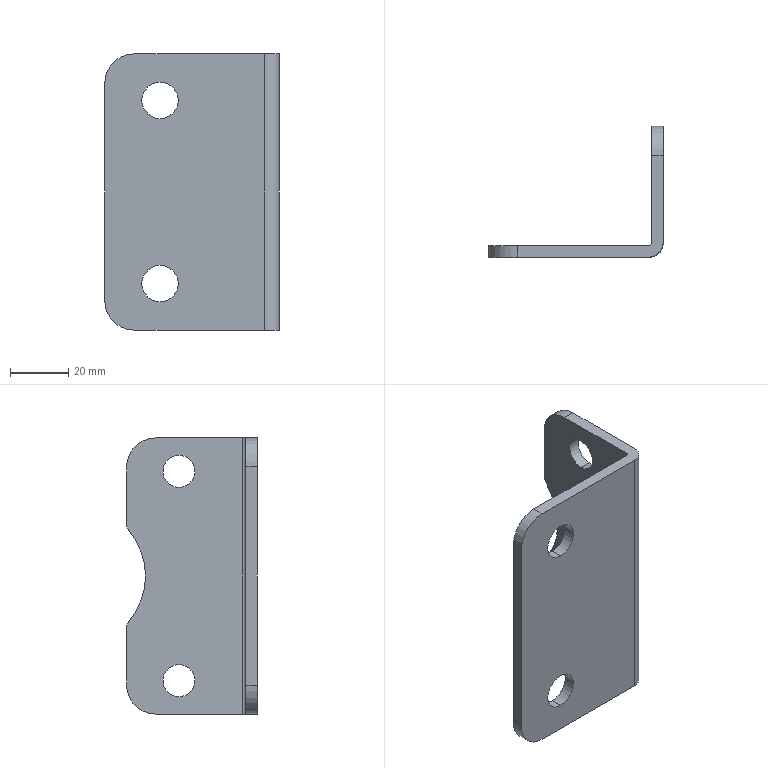Part | NX | features BREP 1 | 1 solid | 26 faces | box 60 x 45 x 95 mm | volume 35211 mm3 | cylinder 17 | plane 9 | commonest cylinder face diameters 11 x4 12.5 x4 20 x4 4 x2 2 x1 10 x1
STEP:
#1=CARTESIAN_POINT('',(-41.,-63.,-37.75));
#2=VERTEX_POINT('',#1);
#3=CARTESIAN_POINT('',(-41.,-63.,-25.25));
#4=VERTEX_POINT('',#3);
#5=CARTESIAN_POINT('',(-41.,-63.,-31.5));
#6=DIRECTION('',(0.,1.,0.));
#7=DIRECTION('',(0.,0.,1.));
#8=AXIS2_PLACEMENT_3D('',#5,#6,#7);
#9=CIRCLE('',#8,6.25);
#10=EDGE_CURVE('',#2,#4,#9,.T.);
#11=ORIENTED_EDGE('',*,*,#10,.F.);
#12=CARTESIAN_POINT('',(-41.,-59.,-37.75));
#13=VERTEX_POINT('',#12);
#14=CARTESIAN_POINT('',(-41.,-59.,-37.75));
#15=DIRECTION('',(0.,1.,0.));
#16=VECTOR('',#15,1000.);
#17=LINE('',#14,#16);
#18=EDGE_CURVE('',#13,#2,#17,.F.);
#19=ORIENTED_EDGE('',*,*,#18,.F.);
#20=CARTESIAN_POINT('',(-41.,-59.,-25.25));
#21=VERTEX_POINT('',#20);
#22=CARTESIAN_POINT('',(-41.,-59.,-31.5));
#23=DIRECTION('',(0.,1.,0.));
#24=DIRECTION('',(0.,0.,1.));
#25=AXIS2_PLACEMENT_3D('',#22,#23,#24);
#26=CIRCLE('',#25,6.25);
#27=EDGE_CURVE('',#13,#21,#26,.T.);
#28=ORIENTED_EDGE('',*,*,#27,.T.);
#29=CARTESIAN_POINT('',(-41.,-59.,-25.25));
#30=DIRECTION('',(0.,1.,0.));
#31=VECTOR('',#30,1000.);
#32=LINE('',#29,#31);
#33=EDGE_CURVE('',#21,#4,#32,.F.);
#34=ORIENTED_EDGE('',*,*,#33,.T.);
#35=EDGE_LOOP('',(#11,#19,#28,#34));
#36=FACE_BOUND('',#35,.T.);
#37=CARTESIAN_POINT('',(-41.,-59.,-31.5));
#38=DIRECTION('',(0.,1.,0.));
#39=DIRECTION('',(0.,0.,1.));
#40=AXIS2_PLACEMENT_3D('',#37,#38,#39);
#41=CYLINDRICAL_SURFACE('',#40,6.25);
#42=ADVANCED_FACE('',(#36),#41,.F.);
#43=CARTESIAN_POINT('',(-41.,-63.,25.25));
#44=VERTEX_POINT('',#43);
#45=CARTESIAN_POINT('',(-41.,-63.,37.75));
#46=VERTEX_POINT('',#45);
#47=CARTESIAN_POINT('',(-41.,-63.,31.5));
#48=DIRECTION('',(0.,1.,0.));
#49=DIRECTION('',(0.,0.,1.));
#50=AXIS2_PLACEMENT_3D('',#47,#48,#49);
#51=CIRCLE('',#50,6.25);
#52=EDGE_CURVE('',#44,#46,#51,.T.);
#53=ORIENTED_EDGE('',*,*,#52,.F.);
#54=CARTESIAN_POINT('',(-41.,-59.,25.25));
#55=VERTEX_POINT('',#54);
#56=CARTESIAN_POINT('',(-41.,-59.,25.25));
#57=DIRECTION('',(0.,1.,0.));
#58=VECTOR('',#57,1000.);
#59=LINE('',#56,#58);
#60=EDGE_CURVE('',#55,#44,#59,.F.);
#61=ORIENTED_EDGE('',*,*,#60,.F.);
#62=CARTESIAN_POINT('',(-41.,-59.,37.75));
#63=VERTEX_POINT('',#62);
#64=CARTESIAN_POINT('',(-41.,-59.,31.5));
#65=DIRECTION('',(0.,1.,0.));
#66=DIRECTION('',(0.,0.,1.));
#67=AXIS2_PLACEMENT_3D('',#64,#65,#66);
#68=CIRCLE('',#67,6.25);
#69=EDGE_CURVE('',#55,#63,#68,.T.);
#70=ORIENTED_EDGE('',*,*,#69,.T.);
#71=CARTESIAN_POINT('',(-41.,-59.,37.75));
#72=DIRECTION('',(0.,1.,0.));
#73=VECTOR('',#72,1000.);
#74=LINE('',#71,#73);
#75=EDGE_CURVE('',#63,#46,#74,.F.);
#76=ORIENTED_EDGE('',*,*,#75,.T.);
#77=EDGE_LOOP('',(#53,#61,#70,#76));
#78=FACE_BOUND('',#77,.T.);
#79=CARTESIAN_POINT('',(-41.,-59.,31.5));
#80=DIRECTION('',(0.,1.,0.));
#81=DIRECTION('',(0.,0.,1.));
#82=AXIS2_PLACEMENT_3D('',#79,#80,#81);
#83=CYLINDRICAL_SURFACE('',#82,6.25);
#84=ADVANCED_FACE('',(#78),#83,.F.);
#85=CARTESIAN_POINT('',(-4.,-36.,-41.5));
#86=VERTEX_POINT('',#85);
#87=CARTESIAN_POINT('',(-4.,-36.,-30.5));
#88=VERTEX_POINT('',#87);
#89=CARTESIAN_POINT('',(-4.,-36.,-36.));
#90=DIRECTION('',(-1.,0.,0.));
#91=DIRECTION('',(0.,0.,-1.));
#92=AXIS2_PLACEMENT_3D('',#89,#90,#91);
#93=CIRCLE('',#92,5.5);
#94=EDGE_CURVE('',#86,#88,#93,.T.);
#95=ORIENTED_EDGE('',*,*,#94,.T.);
#96=CARTESIAN_POINT('',(0.,-36.,-30.5));
#97=VERTEX_POINT('',#96);
#98=CARTESIAN_POINT('',(4.,-36.,-30.5));
#99=DIRECTION('',(1.,0.,0.));
#100=VECTOR('',#99,1000.);
#101=LINE('',#98,#100);
#102=EDGE_CURVE('',#88,#97,#101,.T.);
#103=ORIENTED_EDGE('',*,*,#102,.T.);
#104=CARTESIAN_POINT('',(0.,-36.,-41.5));
#105=VERTEX_POINT('',#104);
#106=CARTESIAN_POINT('',(0.,-36.,-36.));
#107=DIRECTION('',(1.,0.,0.));
#108=DIRECTION('',(0.,0.,-1.));
#109=AXIS2_PLACEMENT_3D('',#106,#107,#108);
#110=CIRCLE('',#109,5.5);
#111=EDGE_CURVE('',#97,#105,#110,.T.);
#112=ORIENTED_EDGE('',*,*,#111,.T.);
#113=CARTESIAN_POINT('',(4.,-36.,-41.5));
#114=DIRECTION('',(1.,0.,0.));
#115=VECTOR('',#114,1000.);
#116=LINE('',#113,#115);
#117=EDGE_CURVE('',#86,#105,#116,.T.);
#118=ORIENTED_EDGE('',*,*,#117,.F.);
#119=EDGE_LOOP('',(#95,#103,#112,#118));
#120=FACE_BOUND('',#119,.T.);
#121=CARTESIAN_POINT('',(4.,-36.,-36.));
#122=DIRECTION('',(1.,0.,0.));
#123=DIRECTION('',(0.,0.,-1.));
#124=AXIS2_PLACEMENT_3D('',#121,#122,#123);
#125=CYLINDRICAL_SURFACE('',#124,5.5);
#126=ADVANCED_FACE('',(#120),#125,.F.);
#127=CARTESIAN_POINT('',(-4.,-36.,30.5));
#128=VERTEX_POINT('',#127);
#129=CARTESIAN_POINT('',(-4.,-36.,41.5));
#130=VERTEX_POINT('',#129);
#131=CARTESIAN_POINT('',(-4.,-36.,36.));
#132=DIRECTION('',(-1.,0.,0.));
#133=DIRECTION('',(0.,0.,-1.));
#134=AXIS2_PLACEMENT_3D('',#131,#132,#133);
#135=CIRCLE('',#134,5.5);
#136=EDGE_CURVE('',#128,#130,#135,.T.);
#137=ORIENTED_EDGE('',*,*,#136,.T.);
#138=CARTESIAN_POINT('',(0.,-36.,41.5));
#139=VERTEX_POINT('',#138);
#140=CARTESIAN_POINT('',(4.,-36.,41.5));
#141=DIRECTION('',(1.,0.,0.));
#142=VECTOR('',#141,1000.);
#143=LINE('',#140,#142);
#144=EDGE_CURVE('',#130,#139,#143,.T.);
#145=ORIENTED_EDGE('',*,*,#144,.T.);
#146=CARTESIAN_POINT('',(0.,-36.,30.5));
#147=VERTEX_POINT('',#146);
#148=CARTESIAN_POINT('',(0.,-36.,36.));
#149=DIRECTION('',(1.,0.,0.));
#150=DIRECTION('',(0.,0.,-1.));
#151=AXIS2_PLACEMENT_3D('',#148,#149,#150);
#152=CIRCLE('',#151,5.5);
#153=EDGE_CURVE('',#139,#147,#152,.T.);
#154=ORIENTED_EDGE('',*,*,#153,.T.);
#155=CARTESIAN_POINT('',(4.,-36.,30.5));
#156=DIRECTION('',(1.,0.,0.));
#157=VECTOR('',#156,1000.);
#158=LINE('',#155,#157);
#159=EDGE_CURVE('',#128,#147,#158,.T.);
#160=ORIENTED_EDGE('',*,*,#159,.F.);
#161=EDGE_LOOP('',(#137,#145,#154,#160));
#162=FACE_BOUND('',#161,.T.);
#163=CARTESIAN_POINT('',(4.,-36.,36.));
#164=DIRECTION('',(1.,0.,0.));
#165=DIRECTION('',(0.,0.,-1.));
#166=AXIS2_PLACEMENT_3D('',#163,#164,#165);
#167=CYLINDRICAL_SURFACE('',#166,5.5);
#168=ADVANCED_FACE('',(#162),#167,.F.);
#169=CARTESIAN_POINT('',(-50.,-59.,47.5));
#170=VERTEX_POINT('',#169);
#171=CARTESIAN_POINT('',(-60.,-59.,37.5));
#172=VERTEX_POINT('',#171);
#173=CARTESIAN_POINT('',(-50.,-59.,37.5));
#174=DIRECTION('',(0.,-1.,0.));
#175=DIRECTION('',(0.,0.,1.));
#176=AXIS2_PLACEMENT_3D('',#173,#174,#175);
#177=CIRCLE('',#176,10.);
#178=EDGE_CURVE('',#170,#172,#177,.T.);
#179=ORIENTED_EDGE('',*,*,#178,.F.);
#180=CARTESIAN_POINT('',(-5.,-59.,47.5));
#181=VERTEX_POINT('',#180);
#182=CARTESIAN_POINT('',(-5.,-59.,47.5));
#183=DIRECTION('',(-1.,0.,0.));
#184=VECTOR('',#183,1000.);
#185=LINE('',#182,#184);
#186=EDGE_CURVE('',#181,#170,#185,.T.);
#187=ORIENTED_EDGE('',*,*,#186,.F.);
#188=CARTESIAN_POINT('',(-5.,-59.,-47.5));
#189=VERTEX_POINT('',#188);
#190=CARTESIAN_POINT('',(-5.,-59.,47.5));
#191=DIRECTION('',(0.,0.,1.));
#192=VECTOR('',#191,1000.);
#193=LINE('',#190,#192);
#194=EDGE_CURVE('',#189,#181,#193,.T.);
#195=ORIENTED_EDGE('',*,*,#194,.F.);
#196=CARTESIAN_POINT('',(-50.,-59.,-47.5));
#197=VERTEX_POINT('',#196);
#198=CARTESIAN_POINT('',(-5.,-59.,-47.5));
#199=DIRECTION('',(1.,0.,0.));
#200=VECTOR('',#199,1000.);
#201=LINE('',#198,#200);
#202=EDGE_CURVE('',#197,#189,#201,.T.);
#203=ORIENTED_EDGE('',*,*,#202,.F.);
#204=CARTESIAN_POINT('',(-60.,-59.,-37.5));
#205=VERTEX_POINT('',#204);
#206=CARTESIAN_POINT('',(-50.,-59.,-37.5));
#207=DIRECTION('',(0.,-1.,0.));
#208=DIRECTION('',(0.,0.,1.));
#209=AXIS2_PLACEMENT_3D('',#206,#207,#208);
#210=CIRCLE('',#209,10.);
#211=EDGE_CURVE('',#205,#197,#210,.T.);
#212=ORIENTED_EDGE('',*,*,#211,.F.);
#213=CARTESIAN_POINT('',(-60.,-59.,47.5));
#214=DIRECTION('',(0.,0.,-1.));
#215=VECTOR('',#214,1000.);
#216=LINE('',#213,#215);
#217=EDGE_CURVE('',#172,#205,#216,.T.);
#218=ORIENTED_EDGE('',*,*,#217,.F.);
#219=EDGE_LOOP('',(#179,#187,#195,#203,#212,#218));
#220=FACE_BOUND('',#219,.T.);
#221=CARTESIAN_POINT('',(-41.,-59.,-31.5));
#222=DIRECTION('',(0.,1.,0.));
#223=DIRECTION('',(0.,0.,1.));
#224=AXIS2_PLACEMENT_3D('',#221,#222,#223);
#225=CIRCLE('',#224,6.25);
#226=EDGE_CURVE('',#21,#13,#225,.T.);
#227=ORIENTED_EDGE('',*,*,#226,.F.);
#228=ORIENTED_EDGE('',*,*,#27,.F.);
#229=EDGE_LOOP('',(#227,#228));
#230=FACE_BOUND('',#229,.T.);
#231=CARTESIAN_POINT('',(-41.,-59.,31.5));
#232=DIRECTION('',(0.,1.,0.));
#233=DIRECTION('',(0.,0.,1.));
#234=AXIS2_PLACEMENT_3D('',#231,#232,#233);
#235=CIRCLE('',#234,6.25);
#236=EDGE_CURVE('',#63,#55,#235,.T.);
#237=ORIENTED_EDGE('',*,*,#236,.F.);
#238=ORIENTED_EDGE('',*,*,#69,.F.);
#239=EDGE_LOOP('',(#237,#238));
#240=FACE_BOUND('',#239,.T.);
#241=CARTESIAN_POINT('',(-5.,-59.,47.5));
#242=DIRECTION('',(0.,-1.,0.));
#243=DIRECTION('',(0.,0.,-1.));
#244=AXIS2_PLACEMENT_3D('',#241,#242,#243);
#245=PLANE('',#244);
#246=ADVANCED_FACE('',(#220,#230,#240),#245,.F.);
#247=CARTESIAN_POINT('',(-60.,-63.,37.5));
#248=VERTEX_POINT('',#247);
#249=CARTESIAN_POINT('',(-60.,-59.,37.5));
#250=DIRECTION('',(0.,-1.,0.));
#251=VECTOR('',#250,1000.);
#252=LINE('',#249,#251);
#253=EDGE_CURVE('',#172,#248,#252,.T.);
#254=ORIENTED_EDGE('',*,*,#253,.F.);
#255=ORIENTED_EDGE('',*,*,#217,.T.);
#256=CARTESIAN_POINT('',(-60.,-63.,-37.5));
#257=VERTEX_POINT('',#256);
#258=CARTESIAN_POINT('',(-60.,-59.,-37.5));
#259=DIRECTION('',(0.,1.,0.));
#260=VECTOR('',#259,1000.);
#261=LINE('',#258,#260);
#262=EDGE_CURVE('',#257,#205,#261,.T.);
#263=ORIENTED_EDGE('',*,*,#262,.F.);
#264=CARTESIAN_POINT('',(-60.,-63.,47.5));
#265=DIRECTION('',(0.,0.,-1.));
#266=VECTOR('',#265,1000.);
#267=LINE('',#264,#266);
#268=EDGE_CURVE('',#248,#257,#267,.T.);
#269=ORIENTED_EDGE('',*,*,#268,.F.);
#270=EDGE_LOOP('',(#254,#255,#263,#269));
#271=FACE_BOUND('',#270,.T.);
#272=CARTESIAN_POINT('',(-60.,-59.,47.5));
#273=DIRECTION('',(1.,0.,0.));
#274=DIRECTION('',(0.,1.,0.));
#275=AXIS2_PLACEMENT_3D('',#272,#273,#274);
#276=PLANE('',#275);
#277=ADVANCED_FACE('',(#271),#276,.F.);
#278=ORIENTED_EDGE('',*,*,#253,.T.);
#279=CARTESIAN_POINT('',(-50.,-63.,47.5));
#280=VERTEX_POINT('',#279);
#281=CARTESIAN_POINT('',(-50.,-63.,37.5));
#282=DIRECTION('',(0.,1.,0.));
#283=DIRECTION('',(0.,0.,1.));
#284=AXIS2_PLACEMENT_3D('',#281,#282,#283);
#285=CIRCLE('',#284,10.);
#286=EDGE_CURVE('',#248,#280,#285,.T.);
#287=ORIENTED_EDGE('',*,*,#286,.T.);
#288=CARTESIAN_POINT('',(-50.,-59.,47.5));
#289=DIRECTION('',(0.,1.,0.));
#290=VECTOR('',#289,1000.);
#291=LINE('',#288,#290);
#292=EDGE_CURVE('',#280,#170,#291,.T.);
#293=ORIENTED_EDGE('',*,*,#292,.T.);
#294=ORIENTED_EDGE('',*,*,#178,.T.);
#295=EDGE_LOOP('',(#278,#287,#293,#294));
#296=FACE_BOUND('',#295,.T.);
#297=CARTESIAN_POINT('',(-50.,-59.,37.5));
#298=DIRECTION('',(0.,1.,0.));
#299=DIRECTION('',(0.,0.,1.));
#300=AXIS2_PLACEMENT_3D('',#297,#298,#299);
#301=CYLINDRICAL_SURFACE('',#300,10.);
#302=ADVANCED_FACE('',(#296),#301,.T.);
#303=ORIENTED_EDGE('',*,*,#186,.T.);
#304=ORIENTED_EDGE('',*,*,#292,.F.);
#305=CARTESIAN_POINT('',(-5.,-63.,47.5));
#306=VERTEX_POINT('',#305);
#307=CARTESIAN_POINT('',(-5.,-63.,47.5));
#308=DIRECTION('',(1.,0.,0.));
#309=VECTOR('',#308,1000.);
#310=LINE('',#307,#309);
#311=EDGE_CURVE('',#280,#306,#310,.T.);
#312=ORIENTED_EDGE('',*,*,#311,.T.);
#313=CARTESIAN_POINT('',(0.,-58.,47.5));
#314=VERTEX_POINT('',#313);
#315=CARTESIAN_POINT('',(-5.,-58.,47.5));
#316=DIRECTION('',(0.,0.,1.));
#317=DIRECTION('',(1.,0.,0.));
#318=AXIS2_PLACEMENT_3D('',#315,#316,#317);
#319=CIRCLE('',#318,5.);
#320=EDGE_CURVE('',#306,#314,#319,.T.);
#321=ORIENTED_EDGE('',*,*,#320,.T.);
#322=CARTESIAN_POINT('',(0.,-28.,47.5));
#323=VERTEX_POINT('',#322);
#324=CARTESIAN_POINT('',(0.,-58.,47.5));
#325=DIRECTION('',(0.,1.,0.));
#326=VECTOR('',#325,1000.);
#327=LINE('',#324,#326);
#328=EDGE_CURVE('',#314,#323,#327,.T.);
#329=ORIENTED_EDGE('',*,*,#328,.T.);
#330=CARTESIAN_POINT('',(-4.,-28.,47.5));
#331=VERTEX_POINT('',#330);
#332=CARTESIAN_POINT('',(-5.,-28.,47.5));
#333=DIRECTION('',(-1.,0.,0.));
#334=VECTOR('',#333,1000.);
#335=LINE('',#332,#334);
#336=EDGE_CURVE('',#323,#331,#335,.T.);
#337=ORIENTED_EDGE('',*,*,#336,.T.);
#338=CARTESIAN_POINT('',(-4.,-58.,47.5));
#339=VERTEX_POINT('',#338);
#340=CARTESIAN_POINT('',(-4.,-58.,47.5));
#341=DIRECTION('',(0.,-1.,0.));
#342=VECTOR('',#341,1000.);
#343=LINE('',#340,#342);
#344=EDGE_CURVE('',#331,#339,#343,.T.);
#345=ORIENTED_EDGE('',*,*,#344,.T.);
#346=CARTESIAN_POINT('',(-5.,-58.,47.5));
#347=DIRECTION('',(0.,0.,-1.));
#348=DIRECTION('',(1.,0.,0.));
#349=AXIS2_PLACEMENT_3D('',#346,#347,#348);
#350=CIRCLE('',#349,1.);
#351=EDGE_CURVE('',#339,#181,#350,.T.);
#352=ORIENTED_EDGE('',*,*,#351,.T.);
#353=EDGE_LOOP('',(#303,#304,#312,#321,#329,#337,#345,#352));
#354=FACE_BOUND('',#353,.T.);
#355=CARTESIAN_POINT('',(-5.,-58.,47.5));
#356=DIRECTION('',(0.,0.,1.));
#357=DIRECTION('',(1.,0.,0.));
#358=AXIS2_PLACEMENT_3D('',#355,#356,#357);
#359=PLANE('',#358);
#360=ADVANCED_FACE('',(#354),#359,.T.);
#361=ORIENTED_EDGE('',*,*,#194,.T.);
#362=ORIENTED_EDGE('',*,*,#351,.F.);
#363=CARTESIAN_POINT('',(-4.,-58.,-47.5));
#364=VERTEX_POINT('',#363);
#365=CARTESIAN_POINT('',(-4.,-58.,47.5));
#366=DIRECTION('',(0.,0.,1.));
#367=VECTOR('',#366,1000.);
#368=LINE('',#365,#367);
#369=EDGE_CURVE('',#364,#339,#368,.T.);
#370=ORIENTED_EDGE('',*,*,#369,.F.);
#371=CARTESIAN_POINT('',(-5.,-58.,-47.5));
#372=DIRECTION('',(0.,0.,1.));
#373=DIRECTION('',(1.,0.,0.));
#374=AXIS2_PLACEMENT_3D('',#371,#372,#373);
#375=CIRCLE('',#374,1.);
#376=EDGE_CURVE('',#189,#364,#375,.T.);
#377=ORIENTED_EDGE('',*,*,#376,.F.);
#378=EDGE_LOOP('',(#361,#362,#370,#377));
#379=FACE_BOUND('',#378,.T.);
#380=CARTESIAN_POINT('',(-5.,-58.,47.5));
#381=DIRECTION('',(0.,0.,1.));
#382=DIRECTION('',(1.,0.,0.));
#383=AXIS2_PLACEMENT_3D('',#380,#381,#382);
#384=CYLINDRICAL_SURFACE('',#383,1.);
#385=ADVANCED_FACE('',(#379),#384,.F.);
#386=CARTESIAN_POINT('',(-50.,-63.,-47.5));
#387=VERTEX_POINT('',#386);
#388=CARTESIAN_POINT('',(-50.,-58.,-47.5));
#389=DIRECTION('',(0.,-1.,0.));
#390=VECTOR('',#389,1000.);
#391=LINE('',#388,#390);
#392=EDGE_CURVE('',#197,#387,#391,.T.);
#393=ORIENTED_EDGE('',*,*,#392,.F.);
#394=ORIENTED_EDGE('',*,*,#202,.T.);
#395=ORIENTED_EDGE('',*,*,#376,.T.);
#396=CARTESIAN_POINT('',(-4.,-28.,-47.5));
#397=VERTEX_POINT('',#396);
#398=CARTESIAN_POINT('',(-4.,-58.,-47.5));
#399=DIRECTION('',(0.,-1.,0.));
#400=VECTOR('',#399,1000.);
#401=LINE('',#398,#400);
#402=EDGE_CURVE('',#397,#364,#401,.T.);
#403=ORIENTED_EDGE('',*,*,#402,.F.);
#404=CARTESIAN_POINT('',(0.,-28.,-47.5));
#405=VERTEX_POINT('',#404);
#406=CARTESIAN_POINT('',(-5.,-28.,-47.5));
#407=DIRECTION('',(-1.,0.,0.));
#408=VECTOR('',#407,1000.);
#409=LINE('',#406,#408);
#410=EDGE_CURVE('',#405,#397,#409,.T.);
#411=ORIENTED_EDGE('',*,*,#410,.F.);
#412=CARTESIAN_POINT('',(0.,-58.,-47.5));
#413=VERTEX_POINT('',#412);
#414=CARTESIAN_POINT('',(0.,-58.,-47.5));
#415=DIRECTION('',(0.,1.,0.));
#416=VECTOR('',#415,1000.);
#417=LINE('',#414,#416);
#418=EDGE_CURVE('',#413,#405,#417,.T.);
#419=ORIENTED_EDGE('',*,*,#418,.F.);
#420=CARTESIAN_POINT('',(-5.,-63.,-47.5));
#421=VERTEX_POINT('',#420);
#422=CARTESIAN_POINT('',(-5.,-58.,-47.5));
#423=DIRECTION('',(0.,0.,1.));
#424=DIRECTION('',(1.,0.,0.));
#425=AXIS2_PLACEMENT_3D('',#422,#423,#424);
#426=CIRCLE('',#425,5.);
#427=EDGE_CURVE('',#421,#413,#426,.T.);
#428=ORIENTED_EDGE('',*,*,#427,.F.);
#429=CARTESIAN_POINT('',(-5.,-63.,-47.5));
#430=DIRECTION('',(1.,0.,0.));
#431=VECTOR('',#430,1000.);
#432=LINE('',#429,#431);
#433=EDGE_CURVE('',#387,#421,#432,.T.);
#434=ORIENTED_EDGE('',*,*,#433,.F.);
#435=EDGE_LOOP('',(#393,#394,#395,#403,#411,#419,#428,#434));
#436=FACE_BOUND('',#435,.T.);
#437=CARTESIAN_POINT('',(-5.,-58.,-47.5));
#438=DIRECTION('',(0.,0.,1.));
#439=DIRECTION('',(1.,0.,0.));
#440=AXIS2_PLACEMENT_3D('',#437,#438,#439);
#441=PLANE('',#440);
#442=ADVANCED_FACE('',(#436),#441,.F.);
#443=ORIENTED_EDGE('',*,*,#392,.T.);
#444=CARTESIAN_POINT('',(-50.,-63.,-37.5));
#445=DIRECTION('',(0.,1.,0.));
#446=DIRECTION('',(0.,0.,1.));
#447=AXIS2_PLACEMENT_3D('',#444,#445,#446);
#448=CIRCLE('',#447,10.);
#449=EDGE_CURVE('',#387,#257,#448,.T.);
#450=ORIENTED_EDGE('',*,*,#449,.T.);
#451=ORIENTED_EDGE('',*,*,#262,.T.);
#452=ORIENTED_EDGE('',*,*,#211,.T.);
#453=EDGE_LOOP('',(#443,#450,#451,#452));
#454=FACE_BOUND('',#453,.T.);
#455=CARTESIAN_POINT('',(-50.,-59.,-37.5));
#456=DIRECTION('',(0.,1.,0.));
#457=DIRECTION('',(0.,0.,1.));
#458=AXIS2_PLACEMENT_3D('',#455,#456,#457);
#459=CYLINDRICAL_SURFACE('',#458,10.);
#460=ADVANCED_FACE('',(#454),#459,.T.);
#461=ORIENTED_EDGE('',*,*,#18,.T.);
#462=CARTESIAN_POINT('',(-41.,-63.,-31.5));
#463=DIRECTION('',(0.,1.,0.));
#464=DIRECTION('',(0.,0.,1.));
#465=AXIS2_PLACEMENT_3D('',#462,#463,#464);
#466=CIRCLE('',#465,6.25);
#467=EDGE_CURVE('',#4,#2,#466,.T.);
#468=ORIENTED_EDGE('',*,*,#467,.F.);
#469=ORIENTED_EDGE('',*,*,#33,.F.);
#470=ORIENTED_EDGE('',*,*,#226,.T.);
#471=EDGE_LOOP('',(#461,#468,#469,#470));
#472=FACE_BOUND('',#471,.T.);
#473=CARTESIAN_POINT('',(-41.,-59.,-31.5));
#474=DIRECTION('',(0.,1.,0.));
#475=DIRECTION('',(0.,0.,1.));
#476=AXIS2_PLACEMENT_3D('',#473,#474,#475);
#477=CYLINDRICAL_SURFACE('',#476,6.25);
#478=ADVANCED_FACE('',(#472),#477,.F.);
#479=ORIENTED_EDGE('',*,*,#60,.T.);
#480=CARTESIAN_POINT('',(-41.,-63.,31.5));
#481=DIRECTION('',(0.,1.,0.));
#482=DIRECTION('',(0.,0.,1.));
#483=AXIS2_PLACEMENT_3D('',#480,#481,#482);
#484=CIRCLE('',#483,6.25);
#485=EDGE_CURVE('',#46,#44,#484,.T.);
#486=ORIENTED_EDGE('',*,*,#485,.F.);
#487=ORIENTED_EDGE('',*,*,#75,.F.);
#488=ORIENTED_EDGE('',*,*,#236,.T.);
#489=EDGE_LOOP('',(#479,#486,#487,#488));
#490=FACE_BOUND('',#489,.T.);
#491=CARTESIAN_POINT('',(-41.,-59.,31.5));
#492=DIRECTION('',(0.,1.,0.));
#493=DIRECTION('',(0.,0.,1.));
#494=AXIS2_PLACEMENT_3D('',#491,#492,#493);
#495=CYLINDRICAL_SURFACE('',#494,6.25);
#496=ADVANCED_FACE('',(#490),#495,.F.);
#497=ORIENTED_EDGE('',*,*,#286,.F.);
#498=ORIENTED_EDGE('',*,*,#268,.T.);
#499=ORIENTED_EDGE('',*,*,#449,.F.);
#500=ORIENTED_EDGE('',*,*,#433,.T.);
#501=CARTESIAN_POINT('',(-5.,-63.,47.5));
#502=DIRECTION('',(0.,0.,-1.));
#503=VECTOR('',#502,1000.);
#504=LINE('',#501,#503);
#505=EDGE_CURVE('',#306,#421,#504,.T.);
#506=ORIENTED_EDGE('',*,*,#505,.F.);
#507=ORIENTED_EDGE('',*,*,#311,.F.);
#508=EDGE_LOOP('',(#497,#498,#499,#500,#506,#507));
#509=FACE_BOUND('',#508,.T.);
#510=ORIENTED_EDGE('',*,*,#467,.T.);
#511=ORIENTED_EDGE('',*,*,#10,.T.);
#512=EDGE_LOOP('',(#510,#511));
#513=FACE_BOUND('',#512,.T.);
#514=ORIENTED_EDGE('',*,*,#485,.T.);
#515=ORIENTED_EDGE('',*,*,#52,.T.);
#516=EDGE_LOOP('',(#514,#515));
#517=FACE_BOUND('',#516,.T.);
#518=CARTESIAN_POINT('',(-60.,-63.,47.5));
#519=DIRECTION('',(0.,1.,0.));
#520=DIRECTION('',(1.,0.,0.));
#521=AXIS2_PLACEMENT_3D('',#518,#519,#520);
#522=PLANE('',#521);
#523=ADVANCED_FACE('',(#509,#513,#517),#522,.F.);
#524=CARTESIAN_POINT('',(-4.,-18.,37.5));
#525=VERTEX_POINT('',#524);
#526=CARTESIAN_POINT('',(-4.,-28.,37.5));
#527=DIRECTION('',(1.,0.,0.));
#528=DIRECTION('',(0.,0.,-1.));
#529=AXIS2_PLACEMENT_3D('',#526,#527,#528);
#530=CIRCLE('',#529,10.);
#531=EDGE_CURVE('',#525,#331,#530,.T.);
#532=ORIENTED_EDGE('',*,*,#531,.F.);
#533=CARTESIAN_POINT('',(-4.,-18.,17.385));
#534=VERTEX_POINT('',#533);
#535=CARTESIAN_POINT('',(-4.,-18.,47.5));
#536=DIRECTION('',(0.,0.,1.));
#537=VECTOR('',#536,1000.);
#538=LINE('',#535,#537);
#539=EDGE_CURVE('',#534,#525,#538,.T.);
#540=ORIENTED_EDGE('',*,*,#539,.F.);
#541=CARTESIAN_POINT('',(-4.,-18.491,16.073));
#542=VERTEX_POINT('',#541);
#543=CARTESIAN_POINT('',(-4.,-20.,17.385));
#544=DIRECTION('',(1.,0.,0.));
#545=DIRECTION('',(0.,0.,-1.));
#546=AXIS2_PLACEMENT_3D('',#543,#544,#545);
#547=CIRCLE('',#546,2.);
#548=EDGE_CURVE('',#542,#534,#547,.T.);
#549=ORIENTED_EDGE('',*,*,#548,.F.);
#550=CARTESIAN_POINT('',(-4.,-18.491,-16.073));
#551=VERTEX_POINT('',#550);
#552=CARTESIAN_POINT('',(-4.,0.,0.));
#553=DIRECTION('',(-1.,0.,0.));
#554=DIRECTION('',(0.,0.,-1.));
#555=AXIS2_PLACEMENT_3D('',#552,#553,#554);
#556=CIRCLE('',#555,24.5);
#557=EDGE_CURVE('',#551,#542,#556,.T.);
#558=ORIENTED_EDGE('',*,*,#557,.F.);
#559=CARTESIAN_POINT('',(-4.,-18.,-17.385));
#560=VERTEX_POINT('',#559);
#561=CARTESIAN_POINT('',(-4.,-20.,-17.385));
#562=DIRECTION('',(1.,0.,0.));
#563=DIRECTION('',(0.,0.,-1.));
#564=AXIS2_PLACEMENT_3D('',#561,#562,#563);
#565=CIRCLE('',#564,2.);
#566=EDGE_CURVE('',#560,#551,#565,.T.);
#567=ORIENTED_EDGE('',*,*,#566,.F.);
#568=CARTESIAN_POINT('',(-4.,-18.,-37.5));
#569=VERTEX_POINT('',#568);
#570=CARTESIAN_POINT('',(-4.,-18.,47.5));
#571=DIRECTION('',(0.,0.,1.));
#572=VECTOR('',#571,1000.);
#573=LINE('',#570,#572);
#574=EDGE_CURVE('',#569,#560,#573,.T.);
#575=ORIENTED_EDGE('',*,*,#574,.F.);
#576=CARTESIAN_POINT('',(-4.,-28.,-37.5));
#577=DIRECTION('',(1.,0.,0.));
#578=DIRECTION('',(0.,0.,-1.));
#579=AXIS2_PLACEMENT_3D('',#576,#577,#578);
#580=CIRCLE('',#579,10.);
#581=EDGE_CURVE('',#397,#569,#580,.T.);
#582=ORIENTED_EDGE('',*,*,#581,.F.);
#583=ORIENTED_EDGE('',*,*,#402,.T.);
#584=ORIENTED_EDGE('',*,*,#369,.T.);
#585=ORIENTED_EDGE('',*,*,#344,.F.);
#586=EDGE_LOOP('',(#532,#540,#549,#558,#567,#575,#582,#583,#584,#585));
#587=FACE_BOUND('',#586,.T.);
#588=ORIENTED_EDGE('',*,*,#94,.F.);
#589=CARTESIAN_POINT('',(-4.,-36.,-36.));
#590=DIRECTION('',(-1.,0.,0.));
#591=DIRECTION('',(0.,0.,-1.));
#592=AXIS2_PLACEMENT_3D('',#589,#590,#591);
#593=CIRCLE('',#592,5.5);
#594=EDGE_CURVE('',#88,#86,#593,.T.);
#595=ORIENTED_EDGE('',*,*,#594,.F.);
#596=EDGE_LOOP('',(#588,#595));
#597=FACE_BOUND('',#596,.T.);
#598=ORIENTED_EDGE('',*,*,#136,.F.);
#599=CARTESIAN_POINT('',(-4.,-36.,36.));
#600=DIRECTION('',(-1.,0.,0.));
#601=DIRECTION('',(0.,0.,-1.));
#602=AXIS2_PLACEMENT_3D('',#599,#600,#601);
#603=CIRCLE('',#602,5.5);
#604=EDGE_CURVE('',#130,#128,#603,.T.);
#605=ORIENTED_EDGE('',*,*,#604,.F.);
#606=EDGE_LOOP('',(#598,#605));
#607=FACE_BOUND('',#606,.T.);
#608=CARTESIAN_POINT('',(-4.,-18.,47.5));
#609=DIRECTION('',(1.,0.,0.));
#610=DIRECTION('',(0.,1.,0.));
#611=AXIS2_PLACEMENT_3D('',#608,#609,#610);
#612=PLANE('',#611);
#613=ADVANCED_FACE('',(#587,#597,#607),#612,.F.);
#614=ORIENTED_EDGE('',*,*,#336,.F.);
#615=CARTESIAN_POINT('',(0.,-18.,37.5));
#616=VERTEX_POINT('',#615);
#617=CARTESIAN_POINT('',(0.,-28.,37.5));
#618=DIRECTION('',(-1.,0.,0.));
#619=DIRECTION('',(0.,0.,-1.));
#620=AXIS2_PLACEMENT_3D('',#617,#618,#619);
#621=CIRCLE('',#620,10.);
#622=EDGE_CURVE('',#323,#616,#621,.T.);
#623=ORIENTED_EDGE('',*,*,#622,.T.);
#624=CARTESIAN_POINT('',(4.,-18.,37.5));
#625=DIRECTION('',(-1.,0.,0.));
#626=VECTOR('',#625,1000.);
#627=LINE('',#624,#626);
#628=EDGE_CURVE('',#616,#525,#627,.T.);
#629=ORIENTED_EDGE('',*,*,#628,.T.);
#630=ORIENTED_EDGE('',*,*,#531,.T.);
#631=EDGE_LOOP('',(#614,#623,#629,#630));
#632=FACE_BOUND('',#631,.T.);
#633=CARTESIAN_POINT('',(4.,-28.,37.5));
#634=DIRECTION('',(1.,0.,0.));
#635=DIRECTION('',(0.,0.,-1.));
#636=AXIS2_PLACEMENT_3D('',#633,#634,#635);
#637=CYLINDRICAL_SURFACE('',#636,10.);
#638=ADVANCED_FACE('',(#632),#637,.T.);
#639=ORIENTED_EDGE('',*,*,#622,.F.);
#640=ORIENTED_EDGE('',*,*,#328,.F.);
#641=CARTESIAN_POINT('',(0.,-58.,47.5));
#642=DIRECTION('',(0.,0.,1.));
#643=VECTOR('',#642,1000.);
#644=LINE('',#641,#643);
#645=EDGE_CURVE('',#413,#314,#644,.T.);
#646=ORIENTED_EDGE('',*,*,#645,.F.);
#647=ORIENTED_EDGE('',*,*,#418,.T.);
#648=CARTESIAN_POINT('',(0.,-18.,-37.5));
#649=VERTEX_POINT('',#648);
#650=CARTESIAN_POINT('',(0.,-28.,-37.5));
#651=DIRECTION('',(-1.,0.,0.));
#652=DIRECTION('',(0.,0.,-1.));
#653=AXIS2_PLACEMENT_3D('',#650,#651,#652);
#654=CIRCLE('',#653,10.);
#655=EDGE_CURVE('',#649,#405,#654,.T.);
#656=ORIENTED_EDGE('',*,*,#655,.F.);
#657=CARTESIAN_POINT('',(0.,-18.,-17.385));
#658=VERTEX_POINT('',#657);
#659=CARTESIAN_POINT('',(0.,-18.,47.5));
#660=DIRECTION('',(0.,0.,-1.));
#661=VECTOR('',#660,1000.);
#662=LINE('',#659,#661);
#663=EDGE_CURVE('',#658,#649,#662,.T.);
#664=ORIENTED_EDGE('',*,*,#663,.F.);
#665=CARTESIAN_POINT('',(0.,-18.491,-16.073));
#666=VERTEX_POINT('',#665);
#667=CARTESIAN_POINT('',(0.,-20.,-17.385));
#668=DIRECTION('',(-1.,0.,0.));
#669=DIRECTION('',(0.,0.,-1.));
#670=AXIS2_PLACEMENT_3D('',#667,#668,#669);
#671=CIRCLE('',#670,2.);
#672=EDGE_CURVE('',#666,#658,#671,.T.);
#673=ORIENTED_EDGE('',*,*,#672,.F.);
#674=CARTESIAN_POINT('',(0.,-18.491,16.073));
#675=VERTEX_POINT('',#674);
#676=CARTESIAN_POINT('',(0.,0.,0.));
#677=DIRECTION('',(1.,0.,0.));
#678=DIRECTION('',(0.,0.,-1.));
#679=AXIS2_PLACEMENT_3D('',#676,#677,#678);
#680=CIRCLE('',#679,24.5);
#681=EDGE_CURVE('',#675,#666,#680,.T.);
#682=ORIENTED_EDGE('',*,*,#681,.F.);
#683=CARTESIAN_POINT('',(0.,-18.,17.385));
#684=VERTEX_POINT('',#683);
#685=CARTESIAN_POINT('',(0.,-20.,17.385));
#686=DIRECTION('',(-1.,0.,0.));
#687=DIRECTION('',(0.,0.,-1.));
#688=AXIS2_PLACEMENT_3D('',#685,#686,#687);
#689=CIRCLE('',#688,2.);
#690=EDGE_CURVE('',#684,#675,#689,.T.);
#691=ORIENTED_EDGE('',*,*,#690,.F.);
#692=CARTESIAN_POINT('',(0.,-18.,47.5));
#693=DIRECTION('',(0.,0.,-1.));
#694=VECTOR('',#693,1000.);
#695=LINE('',#692,#694);
#696=EDGE_CURVE('',#616,#684,#695,.T.);
#697=ORIENTED_EDGE('',*,*,#696,.F.);
#698=EDGE_LOOP('',(#639,#640,#646,#647,#656,#664,#673,#682,#691,#697));
#699=FACE_BOUND('',#698,.T.);
#700=CARTESIAN_POINT('',(0.,-36.,-36.));
#701=DIRECTION('',(1.,0.,0.));
#702=DIRECTION('',(0.,0.,-1.));
#703=AXIS2_PLACEMENT_3D('',#700,#701,#702);
#704=CIRCLE('',#703,5.5);
#705=EDGE_CURVE('',#105,#97,#704,.T.);
#706=ORIENTED_EDGE('',*,*,#705,.F.);
#707=ORIENTED_EDGE('',*,*,#111,.F.);
#708=EDGE_LOOP('',(#706,#707));
#709=FACE_BOUND('',#708,.T.);
#710=CARTESIAN_POINT('',(0.,-36.,36.));
#711=DIRECTION('',(1.,0.,0.));
#712=DIRECTION('',(0.,0.,-1.));
#713=AXIS2_PLACEMENT_3D('',#710,#711,#712);
#714=CIRCLE('',#713,5.5);
#715=EDGE_CURVE('',#147,#139,#714,.T.);
#716=ORIENTED_EDGE('',*,*,#715,.F.);
#717=ORIENTED_EDGE('',*,*,#153,.F.);
#718=EDGE_LOOP('',(#716,#717));
#719=FACE_BOUND('',#718,.T.);
#720=CARTESIAN_POINT('',(0.,-58.,47.5));
#721=DIRECTION('',(-1.,0.,0.));
#722=DIRECTION('',(0.,0.,1.));
#723=AXIS2_PLACEMENT_3D('',#720,#721,#722);
#724=PLANE('',#723);
#725=ADVANCED_FACE('',(#699,#709,#719),#724,.F.);
#726=ORIENTED_EDGE('',*,*,#320,.F.);
#727=ORIENTED_EDGE('',*,*,#505,.T.);
#728=ORIENTED_EDGE('',*,*,#427,.T.);
#729=ORIENTED_EDGE('',*,*,#645,.T.);
#730=EDGE_LOOP('',(#726,#727,#728,#729));
#731=FACE_BOUND('',#730,.T.);
#732=CARTESIAN_POINT('',(-5.,-58.,47.5));
#733=DIRECTION('',(0.,0.,1.));
#734=DIRECTION('',(1.,0.,0.));
#735=AXIS2_PLACEMENT_3D('',#732,#733,#734);
#736=CYLINDRICAL_SURFACE('',#735,5.);
#737=ADVANCED_FACE('',(#731),#736,.T.);
#738=CARTESIAN_POINT('',(4.,-18.,-37.5));
#739=DIRECTION('',(1.,0.,0.));
#740=VECTOR('',#739,1000.);
#741=LINE('',#738,#740);
#742=EDGE_CURVE('',#569,#649,#741,.T.);
#743=ORIENTED_EDGE('',*,*,#742,.T.);
#744=ORIENTED_EDGE('',*,*,#655,.T.);
#745=ORIENTED_EDGE('',*,*,#410,.T.);
#746=ORIENTED_EDGE('',*,*,#581,.T.);
#747=EDGE_LOOP('',(#743,#744,#745,#746));
#748=FACE_BOUND('',#747,.T.);
#749=CARTESIAN_POINT('',(4.,-28.,-37.5));
#750=DIRECTION('',(1.,0.,0.));
#751=DIRECTION('',(0.,0.,-1.));
#752=AXIS2_PLACEMENT_3D('',#749,#750,#751);
#753=CYLINDRICAL_SURFACE('',#752,10.);
#754=ADVANCED_FACE('',(#748),#753,.T.);
#755=ORIENTED_EDGE('',*,*,#628,.F.);
#756=ORIENTED_EDGE('',*,*,#696,.T.);
#757=CARTESIAN_POINT('',(0.,-18.,17.385));
#758=DIRECTION('',(1.,0.,0.));
#759=VECTOR('',#758,1000.);
#760=LINE('',#757,#759);
#761=EDGE_CURVE('',#534,#684,#760,.T.);
#762=ORIENTED_EDGE('',*,*,#761,.F.);
#763=ORIENTED_EDGE('',*,*,#539,.T.);
#764=EDGE_LOOP('',(#755,#756,#762,#763));
#765=FACE_BOUND('',#764,.T.);
#766=CARTESIAN_POINT('',(0.,-18.,47.5));
#767=DIRECTION('',(0.,-1.,0.));
#768=DIRECTION('',(0.,0.,-1.));
#769=AXIS2_PLACEMENT_3D('',#766,#767,#768);
#770=PLANE('',#769);
#771=ADVANCED_FACE('',(#765),#770,.F.);
#772=CARTESIAN_POINT('',(4.,-18.491,-16.073));
#773=DIRECTION('',(1.,0.,0.));
#774=VECTOR('',#773,1000.);
#775=LINE('',#772,#774);
#776=EDGE_CURVE('',#551,#666,#775,.T.);
#777=ORIENTED_EDGE('',*,*,#776,.F.);
#778=ORIENTED_EDGE('',*,*,#557,.T.);
#779=CARTESIAN_POINT('',(4.,-18.491,16.073));
#780=DIRECTION('',(-1.,0.,0.));
#781=VECTOR('',#780,1000.);
#782=LINE('',#779,#781);
#783=EDGE_CURVE('',#675,#542,#782,.T.);
#784=ORIENTED_EDGE('',*,*,#783,.F.);
#785=ORIENTED_EDGE('',*,*,#681,.T.);
#786=EDGE_LOOP('',(#777,#778,#784,#785));
#787=FACE_BOUND('',#786,.T.);
#788=CARTESIAN_POINT('',(4.,0.,0.));
#789=DIRECTION('',(1.,0.,0.));
#790=DIRECTION('',(0.,0.,-1.));
#791=AXIS2_PLACEMENT_3D('',#788,#789,#790);
#792=CYLINDRICAL_SURFACE('',#791,24.5);
#793=ADVANCED_FACE('',(#787),#792,.F.);
#794=CARTESIAN_POINT('',(0.,-18.,-17.385));
#795=DIRECTION('',(-1.,0.,0.));
#796=VECTOR('',#795,1000.);
#797=LINE('',#794,#796);
#798=EDGE_CURVE('',#658,#560,#797,.T.);
#799=ORIENTED_EDGE('',*,*,#798,.F.);
#800=ORIENTED_EDGE('',*,*,#663,.T.);
#801=ORIENTED_EDGE('',*,*,#742,.F.);
#802=ORIENTED_EDGE('',*,*,#574,.T.);
#803=EDGE_LOOP('',(#799,#800,#801,#802));
#804=FACE_BOUND('',#803,.T.);
#805=CARTESIAN_POINT('',(0.,-18.,47.5));
#806=DIRECTION('',(0.,-1.,0.));
#807=DIRECTION('',(0.,0.,-1.));
#808=AXIS2_PLACEMENT_3D('',#805,#806,#807);
#809=PLANE('',#808);
#810=ADVANCED_FACE('',(#804),#809,.F.);
#811=ORIENTED_EDGE('',*,*,#102,.F.);
#812=ORIENTED_EDGE('',*,*,#594,.T.);
#813=ORIENTED_EDGE('',*,*,#117,.T.);
#814=ORIENTED_EDGE('',*,*,#705,.T.);
#815=EDGE_LOOP('',(#811,#812,#813,#814));
#816=FACE_BOUND('',#815,.T.);
#817=CARTESIAN_POINT('',(4.,-36.,-36.));
#818=DIRECTION('',(1.,0.,0.));
#819=DIRECTION('',(0.,0.,-1.));
#820=AXIS2_PLACEMENT_3D('',#817,#818,#819);
#821=CYLINDRICAL_SURFACE('',#820,5.5);
#822=ADVANCED_FACE('',(#816),#821,.F.);
#823=ORIENTED_EDGE('',*,*,#144,.F.);
#824=ORIENTED_EDGE('',*,*,#604,.T.);
#825=ORIENTED_EDGE('',*,*,#159,.T.);
#826=ORIENTED_EDGE('',*,*,#715,.T.);
#827=EDGE_LOOP('',(#823,#824,#825,#826));
#828=FACE_BOUND('',#827,.T.);
#829=CARTESIAN_POINT('',(4.,-36.,36.));
#830=DIRECTION('',(1.,0.,0.));
#831=DIRECTION('',(0.,0.,-1.));
#832=AXIS2_PLACEMENT_3D('',#829,#830,#831);
#833=CYLINDRICAL_SURFACE('',#832,5.5);
#834=ADVANCED_FACE('',(#828),#833,.F.);
#835=ORIENTED_EDGE('',*,*,#761,.T.);
#836=ORIENTED_EDGE('',*,*,#690,.T.);
#837=ORIENTED_EDGE('',*,*,#783,.T.);
#838=ORIENTED_EDGE('',*,*,#548,.T.);
#839=EDGE_LOOP('',(#835,#836,#837,#838));
#840=FACE_BOUND('',#839,.T.);
#841=CARTESIAN_POINT('',(4.,-20.,17.385));
#842=DIRECTION('',(1.,0.,0.));
#843=DIRECTION('',(0.,0.,-1.));
#844=AXIS2_PLACEMENT_3D('',#841,#842,#843);
#845=CYLINDRICAL_SURFACE('',#844,2.);
#846=ADVANCED_FACE('',(#840),#845,.T.);
#847=ORIENTED_EDGE('',*,*,#776,.T.);
#848=ORIENTED_EDGE('',*,*,#672,.T.);
#849=ORIENTED_EDGE('',*,*,#798,.T.);
#850=ORIENTED_EDGE('',*,*,#566,.T.);
#851=EDGE_LOOP('',(#847,#848,#849,#850));
#852=FACE_BOUND('',#851,.T.);
#853=CARTESIAN_POINT('',(4.,-20.,-17.385));
#854=DIRECTION('',(1.,0.,0.));
#855=DIRECTION('',(0.,0.,-1.));
#856=AXIS2_PLACEMENT_3D('',#853,#854,#855);
#857=CYLINDRICAL_SURFACE('',#856,2.);
#858=ADVANCED_FACE('',(#852),#857,.T.);
#859=CLOSED_SHELL('',(#42,#84,#126,#168,#246,#277,#302,#360,#385,#442,#460,#478,#496,#523,#613,#638,#725,#737,#754,#771,#793,#810,#822,#834,#846,#858));
#860=MANIFOLD_SOLID_BREP('',#859);
#861=(LENGTH_UNIT()NAMED_UNIT(*)SI_UNIT(.MILLI.,.METRE.));
#862=UNCERTAINTY_MEASURE_WITH_UNIT(LENGTH_MEASURE(0.00001),#861,'','');
#863=(NAMED_UNIT(*)PLANE_ANGLE_UNIT()SI_UNIT($,.RADIAN.));
#864=(NAMED_UNIT(*)SI_UNIT($,.STERADIAN.)SOLID_ANGLE_UNIT());
#865=(GEOMETRIC_REPRESENTATION_CONTEXT(3)GLOBAL_UNCERTAINTY_ASSIGNED_CONTEXT((#862))GLOBAL_UNIT_ASSIGNED_CONTEXT((#861,#863,#864))REPRESENTATION_CONTEXT('',''));
#866=ADVANCED_BREP_SHAPE_REPRESENTATION('',(#860),#865);